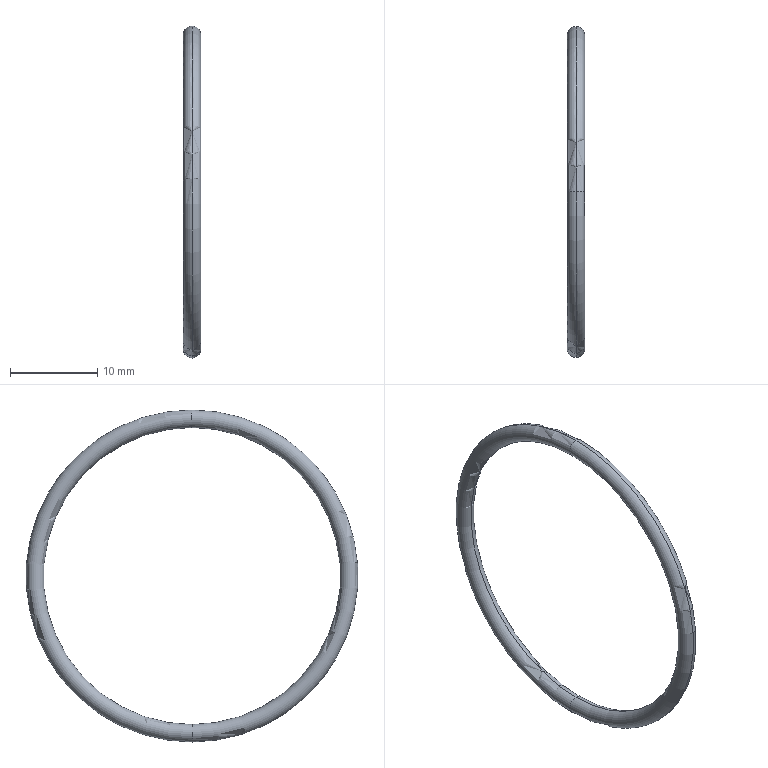Part | SolidWorks | features BaseBody 1 | 1 solid | 4 faces | box 2 x 38 x 38 mm | volume 355.306 mm3 | torus 4
STEP:
#1=CARTESIAN_POINT('',(0.,0.,19.));
#2=VERTEX_POINT('',#1);
#3=CARTESIAN_POINT('',(0.,0.,17.));
#4=VERTEX_POINT('',#3);
#5=CARTESIAN_POINT('',(0.,0.,18.));
#6=DIRECTION('',(0.,1.,0.));
#7=DIRECTION('',(0.,0.,1.));
#8=AXIS2_PLACEMENT_3D('',#5,#6,#7);
#9=CIRCLE('',#8,1.);
#10=EDGE_CURVE('',#2,#4,#9,.T.);
#11=ORIENTED_EDGE('',*,*,#10,.F.);
#12=CARTESIAN_POINT('',(0.,0.,-19.));
#13=VERTEX_POINT('',#12);
#14=CARTESIAN_POINT('',(0.,0.,0.));
#15=DIRECTION('',(1.,0.,0.));
#16=DIRECTION('',(0.,0.,-1.));
#17=AXIS2_PLACEMENT_3D('',#14,#15,#16);
#18=CIRCLE('',#17,19.);
#19=EDGE_CURVE('',#2,#13,#18,.T.);
#20=ORIENTED_EDGE('',*,*,#19,.T.);
#21=CARTESIAN_POINT('',(0.,0.,-17.));
#22=VERTEX_POINT('',#21);
#23=CARTESIAN_POINT('',(0.,0.,-18.));
#24=DIRECTION('',(0.,-1.,0.));
#25=DIRECTION('',(0.,0.,-1.));
#26=AXIS2_PLACEMENT_3D('',#23,#24,#25);
#27=CIRCLE('',#26,1.);
#28=EDGE_CURVE('',#13,#22,#27,.T.);
#29=ORIENTED_EDGE('',*,*,#28,.T.);
#30=CARTESIAN_POINT('',(0.,0.,0.));
#31=DIRECTION('',(1.,0.,0.));
#32=DIRECTION('',(0.,0.,-1.));
#33=AXIS2_PLACEMENT_3D('',#30,#31,#32);
#34=CIRCLE('',#33,17.);
#35=EDGE_CURVE('',#4,#22,#34,.T.);
#36=ORIENTED_EDGE('',*,*,#35,.F.);
#37=EDGE_LOOP('',(#11,#20,#29,#36));
#38=FACE_OUTER_BOUND('',#37,.T.);
#39=CARTESIAN_POINT('',(0.,0.,0.));
#40=DIRECTION('',(1.,0.,0.));
#41=DIRECTION('',(0.,0.,-1.));
#42=AXIS2_PLACEMENT_3D('',#39,#40,#41);
#43=TOROIDAL_SURFACE('',#42,18.,1.);
#44=ADVANCED_FACE('',(#38),#43,.T.);
#45=ORIENTED_EDGE('',*,*,#28,.F.);
#46=CARTESIAN_POINT('',(0.,0.,0.));
#47=DIRECTION('',(1.,0.,0.));
#48=DIRECTION('',(0.,0.,-1.));
#49=AXIS2_PLACEMENT_3D('',#46,#47,#48);
#50=CIRCLE('',#49,19.);
#51=EDGE_CURVE('',#13,#2,#50,.T.);
#52=ORIENTED_EDGE('',*,*,#51,.T.);
#53=ORIENTED_EDGE('',*,*,#10,.T.);
#54=CARTESIAN_POINT('',(0.,0.,0.));
#55=DIRECTION('',(1.,0.,0.));
#56=DIRECTION('',(0.,0.,-1.));
#57=AXIS2_PLACEMENT_3D('',#54,#55,#56);
#58=CIRCLE('',#57,17.);
#59=EDGE_CURVE('',#22,#4,#58,.T.);
#60=ORIENTED_EDGE('',*,*,#59,.F.);
#61=EDGE_LOOP('',(#45,#52,#53,#60));
#62=FACE_OUTER_BOUND('',#61,.T.);
#63=CARTESIAN_POINT('',(0.,0.,0.));
#64=DIRECTION('',(1.,0.,0.));
#65=DIRECTION('',(0.,0.,-1.));
#66=AXIS2_PLACEMENT_3D('',#63,#64,#65);
#67=TOROIDAL_SURFACE('',#66,18.,1.);
#68=ADVANCED_FACE('',(#62),#67,.T.);
#69=ORIENTED_EDGE('',*,*,#51,.F.);
#70=CARTESIAN_POINT('',(0.,0.,-18.));
#71=DIRECTION('',(0.,-1.,0.));
#72=DIRECTION('',(0.,0.,-1.));
#73=AXIS2_PLACEMENT_3D('',#70,#71,#72);
#74=CIRCLE('',#73,1.);
#75=EDGE_CURVE('',#22,#13,#74,.T.);
#76=ORIENTED_EDGE('',*,*,#75,.F.);
#77=ORIENTED_EDGE('',*,*,#59,.T.);
#78=CARTESIAN_POINT('',(0.,0.,18.));
#79=DIRECTION('',(0.,1.,0.));
#80=DIRECTION('',(0.,0.,1.));
#81=AXIS2_PLACEMENT_3D('',#78,#79,#80);
#82=CIRCLE('',#81,1.);
#83=EDGE_CURVE('',#4,#2,#82,.T.);
#84=ORIENTED_EDGE('',*,*,#83,.T.);
#85=EDGE_LOOP('',(#69,#76,#77,#84));
#86=FACE_OUTER_BOUND('',#85,.T.);
#87=CARTESIAN_POINT('',(0.,0.,0.));
#88=DIRECTION('',(1.,0.,0.));
#89=DIRECTION('',(0.,0.,-1.));
#90=AXIS2_PLACEMENT_3D('',#87,#88,#89);
#91=TOROIDAL_SURFACE('',#90,18.,1.);
#92=ADVANCED_FACE('',(#86),#91,.T.);
#93=ORIENTED_EDGE('',*,*,#19,.F.);
#94=ORIENTED_EDGE('',*,*,#83,.F.);
#95=ORIENTED_EDGE('',*,*,#35,.T.);
#96=ORIENTED_EDGE('',*,*,#75,.T.);
#97=EDGE_LOOP('',(#93,#94,#95,#96));
#98=FACE_OUTER_BOUND('',#97,.T.);
#99=CARTESIAN_POINT('',(0.,0.,0.));
#100=DIRECTION('',(1.,0.,0.));
#101=DIRECTION('',(0.,0.,-1.));
#102=AXIS2_PLACEMENT_3D('',#99,#100,#101);
#103=TOROIDAL_SURFACE('',#102,18.,1.);
#104=ADVANCED_FACE('',(#98),#103,.T.);
#105=CLOSED_SHELL('',(#44,#68,#92,#104));
#106=MANIFOLD_SOLID_BREP('',#105);
#107=CARTESIAN_POINT('',(0.,0.,0.));
#108=DIRECTION('',(0.,0.,1.));
#109=DIRECTION('',(1.,0.,0.));
#110=AXIS2_PLACEMENT_3D('',#107,#108,#109);
#111=(LENGTH_UNIT()NAMED_UNIT(*)SI_UNIT(.MILLI.,.METRE.));
#112=UNCERTAINTY_MEASURE_WITH_UNIT(LENGTH_MEASURE(0.00001),#111,'','');
#113=(NAMED_UNIT(*)PLANE_ANGLE_UNIT()SI_UNIT($,.RADIAN.));
#114=(NAMED_UNIT(*)SI_UNIT($,.STERADIAN.)SOLID_ANGLE_UNIT());
#115=(GEOMETRIC_REPRESENTATION_CONTEXT(3)GLOBAL_UNCERTAINTY_ASSIGNED_CONTEXT((#112))GLOBAL_UNIT_ASSIGNED_CONTEXT((#111,#113,#114))REPRESENTATION_CONTEXT('',''));
#116=ADVANCED_BREP_SHAPE_REPRESENTATION('',(#106,#110),#115);